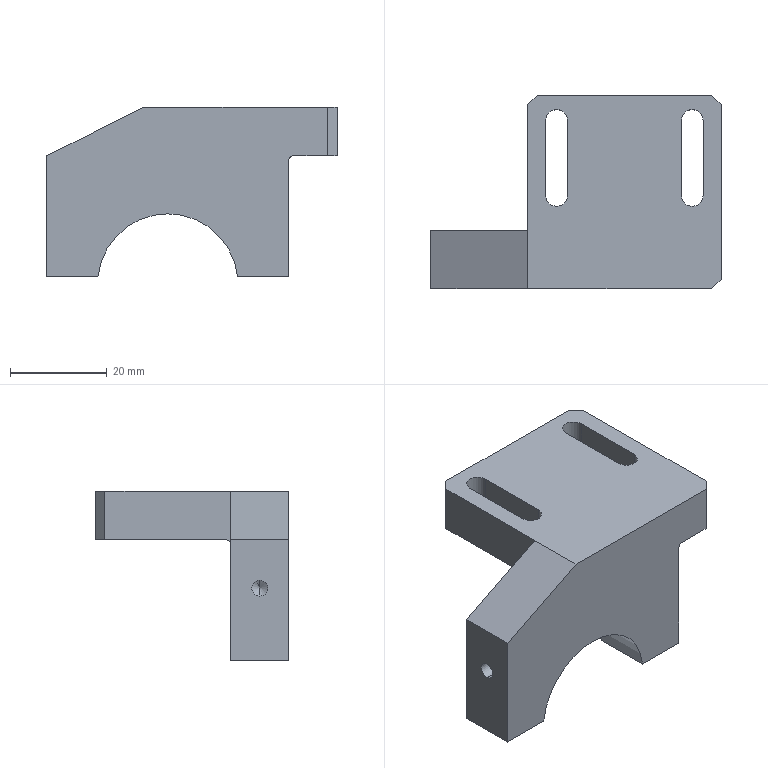NC program | NX | posted with a generic post | part box 60 x 40 x 35 mm
Lines 4653 to 5234 of 5234:
(ZLEVEL_PROFILE_COPY_1 , TOOL : D10JING)
N9304 T14 M6
N9306 G54
N9308 G17 G0 G90 X-5.417 Y10.249 S9500 M3
N9310 G43 Z30. H14
N9312 Z1.5
N9314 G94 G1 Y8. Z1.382 F1000.
N9316 X-5.416 Y7.452 Z1.353
N9318 X-5.742 Y6.138 Z1.282
N9320 X-6.407 Y4.959 Z1.212
N9322 X-7.362 Y4. Z1.141
N9324 X-8.539 Y3.331 Z1.07
N9326 X-9.852 Y3.001 Z0.999
N9328 X-10.4 Y3. Z0.97
N9330 X-30.549 Z-0.086
N9332 X-31.864 Y3.328 Z-0.157
N9334 X-33.045 Y3.996 Z-0.228
N9336 X-34.004 Y4.955 Z-0.299
N9338 X-34.672 Y6.136 Z-0.37
N9340 X-35. Y7.451 Z-0.441
N9342 Y8. Z-0.47
N9344 Y20. Z-1.099
N9346 Y20.549 Z-1.128
N9348 X-34.672 Y21.864 Z-1.199
N9350 X-34.004 Y23.045 Z-1.27
N9352 X-33.045 Y24.004 Z-1.341
N9354 X-31.864 Y24.672 Z-1.412
N9356 X-30.549 Y25. Z-1.483
N9358 X-10.4 Z-2.539
N9360 X-9.852 Y24.999 Z-2.568
N9362 X-8.539 Y24.669 Z-2.639
N9364 X-7.362 Y24. Z-2.71
N9366 X-6.407 Y23.041 Z-2.781
N9368 X-5.742 Y21.862 Z-2.852
N9370 X-5.416 Y20.548 Z-2.923
N9372 X-5.417 Y20. Z-2.951
N9374 Y8. Z-3.58
N9376 X-5.416 Y7.452 Z-3.609
N9378 X-5.742 Y6.138 Z-3.68
N9380 X-6.407 Y4.959 Z-3.751
N9382 X-7.362 Y4. Z-3.822
N9384 X-8.539 Y3.331 Z-3.893
N9386 X-9.852 Y3.001 Z-3.964
N9388 X-10.4 Y3. Z-3.992
N9390 X-30.549 Z-5.048
N9392 X-31.864 Y3.328 Z-5.119
N9394 X-33.045 Y3.996 Z-5.19
N9396 X-34.004 Y4.955 Z-5.261
N9398 X-34.672 Y6.136 Z-5.333
N9400 X-35. Y7.451 Z-5.404
N9402 Y8. Z-5.432
N9404 Y20. Z-6.061
N9406 Y20.549 Z-6.09
N9408 X-34.672 Y21.864 Z-6.161
N9410 X-34.004 Y23.045 Z-6.232
N9412 X-33.045 Y24.004 Z-6.303
N9414 X-31.864 Y24.672 Z-6.374
N9416 X-30.549 Y25. Z-6.445
N9418 X-10.4 Z-7.501
N9420 X-9.852 Y24.999 Z-7.53
N9422 X-8.539 Y24.669 Z-7.601
N9424 X-7.362 Y24. Z-7.672
N9426 X-6.407 Y23.041 Z-7.743
N9428 X-5.742 Y21.862 Z-7.814
N9430 X-5.416 Y20.548 Z-7.885
N9432 X-5.417 Y20. Z-7.914
N9434 Y8. Z-8.542
N9436 X-5.416 Y7.452 Z-8.571
N9438 X-5.742 Y6.138 Z-8.642
N9440 X-6.407 Y4.959 Z-8.713
N9442 X-7.362 Y4. Z-8.784
N9444 X-8.539 Y3.331 Z-8.855
N9446 X-9.852 Y3.001 Z-8.926
N9448 X-10.4 Y3. Z-8.955
N9450 X-30.549 Z-10.011
N9452 X-31.864 Y3.328 Z-10.082
N9454 X-33.045 Y3.996 Z-10.153
N9456 X-34.004 Y4.955 Z-10.224
N9458 X-34.672 Y6.136 Z-10.295
N9460 X-35. Y7.451 Z-10.366
N9462 Y8. Z-10.395
N9464 Y20. Z-11.024
N9466 Y20.549 Z-11.052
N9468 X-34.672 Y21.864 Z-11.123
N9470 X-34.004 Y23.045 Z-11.194
N9472 X-33.045 Y24.004 Z-11.266
N9474 X-31.864 Y24.672 Z-11.337
N9476 X-30.549 Y25. Z-11.408
N9478 X-20.2 Z-11.95
N9480 X-10.4 F1200.
N9482 G2 X-5.417 Y20. R4.991
N9484 G1 Y8.
N9486 G2 X-10.4 Y3. R4.991
N9488 G1 X-30.
N9490 G2 X-35. Y8. R5.
N9492 G1 Y20.
N9494 G2 X-30. Y25. R5.
N9496 G1 X-20.2
N9498 Z-10.45
N9500 G0 Z30.
N9502 X25. Y10.263
N9504 Z1.5
N9506 G1 Y7.451 Z1.353 F1000.
N9508 X24.672 Y6.136 Z1.282
N9510 X24.004 Y4.955 Z1.211
N9512 X23.045 Y3.996 Z1.139
N9514 X21.864 Y3.328 Z1.068
N9516 X20.549 Y3. Z0.997
N9518 X0.4 Z-0.059
N9520 X-0.148 Y3.001 Z-0.087
N9522 X-1.461 Y3.331 Z-0.158
N9524 X-2.638 Y4. Z-0.229
N9526 X-3.593 Y4.959 Z-0.3
N9528 X-4.258 Y6.138 Z-0.371
N9530 X-4.584 Y7.452 Z-0.442
N9532 X-4.583 Y8. Z-0.471
N9534 Y20. Z-1.1
N9536 X-4.584 Y20.548 Z-1.128
N9538 X-4.258 Y21.862 Z-1.199
N9540 X-3.593 Y23.041 Z-1.27
N9542 X-2.638 Y24. Z-1.341
N9544 X-1.461 Y24.669 Z-1.412
N9546 X-0.148 Y24.999 Z-1.483
N9548 X0.4 Y25. Z-1.512
N9550 X20.549 Z-2.568
N9552 X21.864 Y24.672 Z-2.639
N9554 X23.045 Y24.004 Z-2.71
N9556 X24.004 Y23.045 Z-2.781
N9558 X24.672 Y21.864 Z-2.852
N9560 X25. Y20.549 Z-2.923
N9562 Y20. Z-2.952
N9564 Y7.451 Z-3.61
N9566 X24.672 Y6.136 Z-3.681
N9568 X24.004 Y4.955 Z-3.752
N9570 X23.045 Y3.996 Z-3.823
N9572 X21.864 Y3.328 Z-3.894
N9574 X20.549 Y3. Z-3.965
N9576 X0.4 Z-5.021
N9578 X-0.148 Y3.001 Z-5.05
N9580 X-1.461 Y3.331 Z-5.121
N9582 X-2.638 Y4. Z-5.192
N9584 X-3.593 Y4.959 Z-5.262
N9586 X-4.258 Y6.138 Z-5.333
N9588 X-4.584 Y7.452 Z-5.404
N9590 X-4.583 Y8. Z-5.433
N9592 Y20. Z-6.062
N9594 X-4.584 Y20.548 Z-6.091
N9596 X-4.258 Y21.862 Z-6.162
N9598 X-3.593 Y23.041 Z-6.233
N9600 X-2.638 Y24. Z-6.304
N9602 X-1.461 Y24.669 Z-6.374
N9604 X-0.148 Y24.999 Z-6.445
N9606 X0.4 Y25. Z-6.474
N9608 X20.549 Z-7.53
N9610 X21.864 Y24.672 Z-7.601
N9612 X23.045 Y24.004 Z-7.672
N9614 X24.004 Y23.045 Z-7.743
N9616 X24.672 Y21.864 Z-7.814
N9618 X25. Y20.549 Z-7.885
N9620 Y20. Z-7.914
N9622 Y7.451 Z-8.572
N9624 X24.672 Y6.136 Z-8.643
N9626 X24.004 Y4.955 Z-8.714
N9628 X23.045 Y3.996 Z-8.785
N9630 X21.864 Y3.328 Z-8.856
N9632 X20.549 Y3. Z-8.927
N9634 X0.4 Z-9.983
N9636 X-0.148 Y3.001 Z-10.012
N9638 X-1.461 Y3.331 Z-10.083
N9640 X-2.638 Y4. Z-10.154
N9642 X-3.593 Y4.959 Z-10.225
N9644 X-4.258 Y6.138 Z-10.296
N9646 X-4.584 Y7.452 Z-10.367
N9648 X-4.583 Y8. Z-10.395
N9650 Y20. Z-11.024
N9652 X-4.584 Y20.548 Z-11.053
N9654 X-4.258 Y21.862 Z-11.124
N9656 X-3.593 Y23.041 Z-11.195
N9658 X-2.638 Y24. Z-11.266
N9660 X-1.461 Y24.669 Z-11.337
N9662 X-0.148 Y24.999 Z-11.408
N9664 X0.4 Y25. Z-11.436
N9666 X10.2 Z-11.95
N9668 X20. F1200.
N9670 G2 X25. Y20. R5.
N9672 G1 Y8.
N9674 G2 X20. Y3. R5.
N9676 G1 X0.4
N9678 G2 X-4.583 Y8. R4.991
N9680 G1 Y20.
N9682 G2 X0.4 Y25. R4.991
N9684 G1 X10.2
N9686 X20. Z-12.792
N9688 X20.49 Y24.976 Z-12.834
N9690 X20.975 Y24.904 Z-12.876
N9692 X21.451 Y24.785 Z-12.918
N9694 X21.913 Y24.619 Z-12.96
N9696 X22.357 Y24.41 Z-13.002
N9698 X22.778 Y24.157 Z-13.044
N9700 X23.172 Y23.865 Z-13.086
N9702 X23.536 Y23.536 Z-13.128
N9704 X23.865 Y23.172 Z-13.17
N9706 X24.157 Y22.778 Z-13.212
N9708 X24.41 Y22.357 Z-13.254
N9710 X24.619 Y21.913 Z-13.297
N9712 X24.785 Y21.451 Z-13.339
N9714 X24.904 Y20.975 Z-13.381
N9716 X24.976 Y20.49 Z-13.423
N9718 X25. Y20. Z-13.465
N9720 Y8. Z-14.495
N9722 X24.976 Y7.51 Z-14.537
N9724 X24.904 Y7.025 Z-14.58
N9726 X24.785 Y6.549 Z-14.622
N9728 X24.619 Y6.087 Z-14.664
N9730 X24.41 Y5.643 Z-14.706
N9732 X24.157 Y5.222 Z-14.748
N9734 X23.865 Y4.828 Z-14.79
N9736 X23.536 Y4.464 Z-14.832
N9738 X23.172 Y4.135 Z-14.874
N9740 X22.778 Y3.843 Z-14.916
N9742 X22.357 Y3.59 Z-14.958
N9744 X21.913 Y3.381 Z-15.
N9746 X21.451 Y3.215 Z-15.042
N9748 X20.975 Y3.096 Z-15.085
N9750 X20.49 Y3.024 Z-15.127
N9752 X20. Y3. Z-15.169
N9754 X0.397 Z-16.852
N9756 X-0.573 Z-16.935
N9758 X-1.509 Z-17.016
N9760 X-2.371 Z-17.092
N9762 X-3.127 Z-17.16
N9764 X-3.746 Z-17.217
N9766 X-4.206 Z-17.264
N9768 X-4.488 Z-17.299
N9770 X-4.583 Z-17.325
N9772 X-13.055 Z-17.831
N9774 X-21.528 Z-18.356
N9776 X-30. Z-18.901
N9778 X-30.569 Y3.032 Z-18.933
N9780 X-30.975 Y3.096 Z-18.965
N9782 X-31.496 Y3.229 Z-18.998
N9784 X-31.913 Y3.381 Z-19.03
N9786 X-32.385 Y3.605 Z-19.062
N9788 X-32.778 Y3.843 Z-19.094
N9790 X-33.189 Y4.149 Z-19.126
N9792 X-33.536 Y4.464 Z-19.158
N9794 X-33.875 Y4.84 Z-19.19
N9796 X-34.157 Y5.222 Z-19.222
N9798 X-34.415 Y5.652 Z-19.253
N9800 X-34.619 Y6.087 Z-19.285
N9802 X-34.786 Y6.554 Z-19.316
N9804 X-34.904 Y7.025 Z-19.348
N9806 X-34.976 Y7.512 Z-19.379
N9808 X-35. Y8. Z-19.41
N9810 Y20. Z-20.434
N9812 X-34.976 Y20.488 Z-20.465
N9814 X-34.904 Y20.975 Z-20.497
N9816 X-34.786 Y21.446 Z-20.528
N9818 X-34.619 Y21.913 Z-20.56
N9820 X-34.415 Y22.348 Z-20.591
N9822 X-34.157 Y22.778 Z-20.622
N9824 X-33.875 Y23.16 Z-20.653
N9826 X-33.536 Y23.536 Z-20.684
N9828 X-33.189 Y23.851 Z-20.715
N9830 X-32.778 Y24.157 Z-20.745
N9832 X-32.385 Y24.395 Z-20.776
N9834 X-31.913 Y24.619 Z-20.806
N9836 X-31.496 Y24.771 Z-20.837
N9838 X-30.975 Y24.904 Z-20.868
N9840 X-30.569 Y24.968 Z-20.898
N9842 X-30. Y25. Z-20.929
N9844 X-21.528 Z-21.467
N9846 X-13.055 Z-22.024
N9848 X-4.583 Z-22.602
N9850 X-4.488 Z-22.625
N9852 X-4.206 Z-22.656
N9854 X-3.746 Z-22.699
N9856 X-3.127 Z-22.754
N9858 X-2.371 Z-22.82
N9860 X-1.509 Z-22.894
N9862 X-0.573 Z-22.975
N9864 X0.397 Z-23.058
N9866 X10.2 Z-23.9
N9868 X20.
N9870 G2 X25. Y20. R5.
N9872 G1 Y8.
N9874 G2 X20. Y3. R5.
N9876 G1 X-30.
N9878 G2 X-35. Y8. R5.
N9880 G1 Y20.
N9882 G2 X-30. Y25. R5.
N9884 G1 X10.2
N9886 Z-22.4
N9888 G0 Z30.
(ZLEVEL_PROFILE_COPY_1_COPY , TOOL : D10JING)
N9890 X5.442
N9892 Z-23.5
N9894 G1 X28.549 Z-24.711 F1000.
N9896 X29.925 Y24.647 Z-24.785
N9898 X31.148 Y23.923 Z-24.86
N9900 X33.923 Y21.148 Z-25.066
N9902 X34.647 Y19.925 Z-25.14
N9904 X35. Y18.549 Z-25.215
N9906 Y18. Z-25.243
N9908 Y-18. Z-27.13
N9910 Y-18.549 Z-27.159
N9912 X34.647 Y-19.925 Z-27.233
N9914 X33.923 Y-21.148 Z-27.308
N9916 X31.148 Y-23.923 Z-27.513
N9918 X29.925 Y-24.647 Z-27.588
N9920 X28.549 Y-25. Z-27.662
N9922 X-8.549 Z-29.607
N9924 X-9.925 Y-24.647 Z-29.681
N9926 X-11.148 Y-23.923 Z-29.755
N9928 X-13.536 Y-21.536 Z-29.932
N9930 X-13.923 Y-21.148 Z-29.961
N9932 X-14.647 Y-19.925 Z-30.036
N9934 X-15. Y-18.549 Z-30.11
N9936 Y3. Z-31.239
N9938 X-30.549 Z-32.054
N9940 X-31.864 Y3.328 Z-32.125
N9942 X-33.045 Y3.996 Z-32.196
N9944 X-34.004 Y4.955 Z-32.268
N9946 X-34.672 Y6.136 Z-32.339
N9948 X-35. Y7.451 Z-32.41
N9950 Y20.549 Z-33.096
N9952 X-34.672 Y21.864 Z-33.167
N9954 X-34.004 Y23.045 Z-33.238
N9956 X-33.045 Y24.004 Z-33.309
N9958 X-31.864 Y24.672 Z-33.38
N9960 X-30.549 Y25. Z-33.451
N9962 X-1. Z-35.
N9964 X28. F1200.
N9966 G2 X31.536 Y23.536 R5.
N9968 G1 X33.536 Y21.536
N9970 G2 X35. Y18. R5.
N9972 G1 Y-18.
N9974 G2 X33.536 Y-21.536 R5.
N9976 G1 X31.536 Y-23.536
N9978 G2 X28. Y-25. R5.
N9980 G1 X-8.
N9982 G2 X-11.536 Y-23.536 R5.
N9984 G1 X-13.536 Y-21.536
N9986 G2 X-15. Y-18. R5.
N9988 G1 Y3.
N9990 X-30.
N9992 G2 X-35. Y8. R5.
N9994 G1 Y20.
N9996 G2 X-30. Y25. R5.
N9998 G1 X-1.
N10000 Z-33.5
N10002 G0 Z30.
(ZLEVEL_PROFILE_1 , TOOL : D6R0.5)
N10004 T16 M6
N10006 G17 G43 G0 G90 X23.543 Y23.632 Z30. S7500 H16 M3
N10008 Z-23.1
N10010 G94 G1 Z-24.1 F2000.
N10012 X23.299 Y23.491
N10014 G3 X22.999 Y22.971 R0.6
N10016 G1 X23. Y7.996
N10018 G2 X19.981 Y5. R3.
N10020 G1 X-13.001
N10022 Z-24.2
N10024 X19.981
N10026 G3 X23. Y7.996 R3.
N10028 G1 X22.999 Y22.978
N10030 Y22.985 Z-24.3
N10032 X23. Y7.996
N10034 G2 X19.981 Y5. R3.
N10036 G1 X-13.001
N10038 Z-24.4
N10040 X19.981
N10042 G3 X23. Y7.996 R3.
N10044 G1 X22.999 Y22.992
N10046 X23.007 Y22.999 Z-24.487
N10048 G3 X23. Y7.996 R8478.189
N10050 G2 X20.053 Y5. R3.
N10052 G1 X-10.362 Y4.999
N10054 X-12.991 Y4.99
N10056 Y4.987 Z-24.497
N10058 X-10.362 Y4.998
N10060 X20.001 Y5.002
N10062 G3 X23.001 Y8.001 R3.
N10064 G1 X23. Y19.903
N10066 X23.007 Y20.38
N10068 X23.009 Y22.999
N10070 X23.012 Y23. Z-24.507
N10072 X23.013 Y22.789
N10074 X23.008 Y20.38
N10076 X23. Y19.903
N10078 Y8.34
N10080 X23.002 Y7.998
N10082 G2 X19.981 Y4.999 R2.996
N10084 G1 X-9.673 Y5.
N10086 X-10. Y4.996
N10088 X-12.996 Y4.984
N10090 Y4.98 Z-24.517
N10092 X-11.052 Y4.992
N10094 X-10.707 Y4.996
N10096 X-10. Y4.995
N10098 X8.947 Y5.
N10100 X20.015 Y4.999
N10102 G3 X23. Y7.984 R2.985
N10104 G1 Y19.903
N10106 G3 X23.015 Y23.001 R136.454
N10108 G1 X23.017 Z-24.527
N10110 G2 X23.001 Y19.903 R112.342
N10112 G1 Y7.998
N10114 G2 X20.053 Y4.996 R2.991
N10116 G1 X19.981 Y4.999
N10118 X19.636
N10120 X-10.
N10122 X-10.017 Y4.993
N10124 X-10.362 Y4.992
N10126 X-12.996 Y4.977
N10128 Y4.973 Z-24.537
N10130 G3 X-10.017 Y4.991 R3393.793
N10132 G1 X-10. Y4.999
N10134 X19.636
N10136 X19.981 Y4.998
N10138 X20.053 Y4.995
N10140 G3 X23.001 Y7.997 R2.989
N10142 G1 Y19.903
N10144 G3 X23.021 Y23. R102.309
N10146 G1 X23.035 Z-24.57
N10148 G2 X23.014 Y20.036 R97.428
N10150 G1 X23.005 Y20.
N10152 Y7.996
N10154 G2 X22.828 Y6.964 R2.685
N10156 X20.013 Y4.995 R2.972
N10158 G1 X-10.
N10160 X-10.017 Y4.986
N10162 G3 X-11.397 Y4.966 R36.272
N10164 G1 X-12.996 Y4.96
N10166 Y4.942 Z-24.614
N10168 X-12.997 Y4.925 Z-24.658
N10170 G3 X-10.017 Y4.965 R70.843
N10172 G1 X-10. Y4.974
N10174 X20.053
N10176 G3 X23.026 Y7.947 R2.946
N10178 G1 Y19.812
N10180 G3 X23.071 Y23. R59.216
N10182 G1 X23.089 Z-24.695
N10184 X23.114 Z-24.733
N10186 X23.117 Y22.789
N10188 X23.115 Y21.412
N10190 G3 X23.057 Y19.792 R571.944
N10192 G1 Y7.843
N10194 G2 X20.326 Y4.945 R2.904
N10196 G1 X20.196 Y4.933
N10198 X20.118 Y4.943
N10200 X-10.
N10202 G2 X-12.999 Y4.891 R40.858
N10204 G1 Y4.867 Z-24.764
N10206 Y4.841 Z-24.796
N10208 G3 X-9.804 Y4.903 R46.313
N10210 G1 X20.196
N10212 G3 X23.097 Y7.804 R2.845
N10214 G1 Y19.804
N10216 G3 X23.157 Y22.999 R45.518
N10218 G1 X23.178 Z-24.822
N10220 X23.212 Z-24.849
N10222 G2 X23.142 Y19.864 R39.548
N10224 G1 Y7.717
N10226 X23.148 Y7.701
N10228 X23.132 Y7.464
N10230 G2 X20.345 Y4.858 R2.793
N10232 G1 X-10.
N10234 G2 X-12.998 Y4.79 R34.036
N10236 G1 Y4.763 Z-24.867
N10238 X-12.997 Y4.74 Z-24.886
N10240 G3 X-10. Y4.817 R29.153
N10242 G1 X20.367
N10244 G3 X23.183 Y7.633 R2.75
N10246 G1 Y19.692
N10248 G3 X23.261 Y22.999 R40.684
N10250 G1 X23.294 Z-24.905
N10252 X23.341 Y23. Z-24.923
N10254 G2 X23.233 Y19.756 R32.956
N10256 G1 Y7.531
N10258 G2 X20.47 Y4.767 R2.705
N10260 G1 X-9.742
N10262 G2 X-12.997 Y4.667 R31.849
N10264 G1 Y4.638 Z-24.937
N10266 Y4.604 Z-24.951
N10268 G3 X-9.722 Y4.716 R25.342
N10270 G1 X20.643
N10272 G3 X23.284 Y7.357 R2.641
N10274 G1 Y19.779
N10276 G3 X23.403 Y23. R28.08
N10278 G1 X23.44 Y22.995 Z-24.967
N10280 G2 X23.32 Y19.761 R30.469
N10282 G1 Y7.298
N10284 G2 X20.702 Y4.68 R2.618
N10286 G1 X-9.696
N10288 G2 X-10.657 Y4.592 R8.204
N10290 G1 X-11.397 Y4.569
N10292 X-12.997
N10294 X-12.979 Y4.516 Z-24.981
N10296 G3 X-10.017 Y4.594 R22.414
N10298 G1 X-10. Y4.638
N10300 X20.728
N10302 G3 X23.362 Y7.272 R2.577
N10304 G1 Y19.768
N10306 G3 X23.497 Y22.973 R44.744
N10308 G1 X23.574 Y22.938 Z-25.
N10310 G3 X23.449 Y7.077 R784.906
N10312 G2 X20.924 Y4.547 R2.524
N10314 G1 X-9.328
N10316 G2 X-12.929 Y4.426 R18.993
N10318 G3 X-13.466 Y4.158 R0.6
N10320 G1 X-13.628 Y3.913
N10322 Z-24.
N10324 G0 Z30.
N10326 M5
(PLANAR_MILL_COPY_COPY_COPY_COPY , TOOL : D6A45)
N10328 T01 M6
N10330 G54
N10332 G17 G0 G90 X25.9 Y-8.27 S9500 M3
N10334 G43 Z30. H1
N10336 Z-24.5
N10338 G94 G1 Z-26. F1250.
N10340 X26.6 Y-7.866
N10342 G3 X27.1 Y-7. R1.
N10344 G1 Y0.75
N10346 G3 X24. Y3.85 R3.1
N10348 X20.9 Y0.75 R3.1
N10350 G1 Y-14.75
N10352 G3 X24. Y-17.85 R3.1
N10354 X27.1 Y-14.75 R3.1
N10356 G1 Y-7.
N10358 G3 X26.6 Y-6.134 R1.
N10360 G1 X25.9 Y-5.73
N10362 Z-24.5
N10364 G0 Z30.
N10366 X-4.161 Y2.3
N10368 Z-24.5
N10370 G1 Z-26.
N10372 X-4.565 Y3.
N10374 G3 X-5.431 Y3.5 R1.
N10376 X-7.1 Y0.75 R3.1
N10378 G1 Y-14.75
N10380 G3 X-4. Y-17.85 R3.1
N10382 X-0.9 Y-14.75 R3.1
N10384 G1 Y0.75
N10386 G3 X-2.569 Y3.5 R3.1
N10388 X-3.435 Y3. R1.
N10390 G1 X-3.839 Y2.3
N10392 Z-24.5
N10394 G0 Z30.
N10396 X25.092 Y22.313
N10398 Z-24.5
N10400 G1 Z-26.
N10402 X24.643 Y21.865
N10404 G3 X24.382 Y20.9 R1.
N10406 G1 X27.959
N10408 G2 X28.666 Y20.607 R1.
N10410 G1 X30.607 Y18.666
N10412 G2 X30.9 Y17.959 R1.
N10414 G1 Y-17.959
N10416 G2 X30.607 Y-18.666 R1.
N10418 G1 X28.666 Y-20.607
N10420 G2 X27.959 Y-20.9 R1.
N10422 G1 X-7.959
N10424 G2 X-8.666 Y-20.607 R1.
N10426 G1 X-10.607 Y-18.666
N10428 G2 X-10.9 Y-17.959 R1.
N10430 G1 Y3.618
N10432 G3 X-11.865 Y3.357 R1.
N10434 G1 X-12.313 Y2.908
N10436 Z-24.5
N10438 G0 Z30.
N10440 M5
N10442 M2